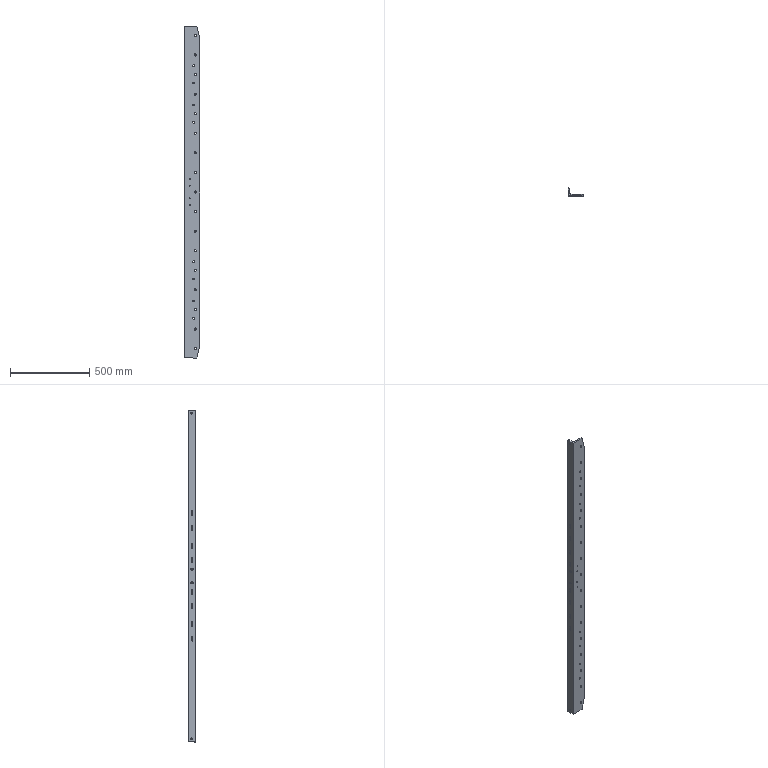Part | SolidWorks | features Fillet 2, ICE 2, Extrusion 1 | 1 solid | 117 faces | box 100 x 50 x 2100 mm | volume 2805771 mm3 | cylinder 93 | plane 24 | commonest cylinder face diameters 13 x38 10.5 x24 11 x20 7 x8 20 x2 16 x1